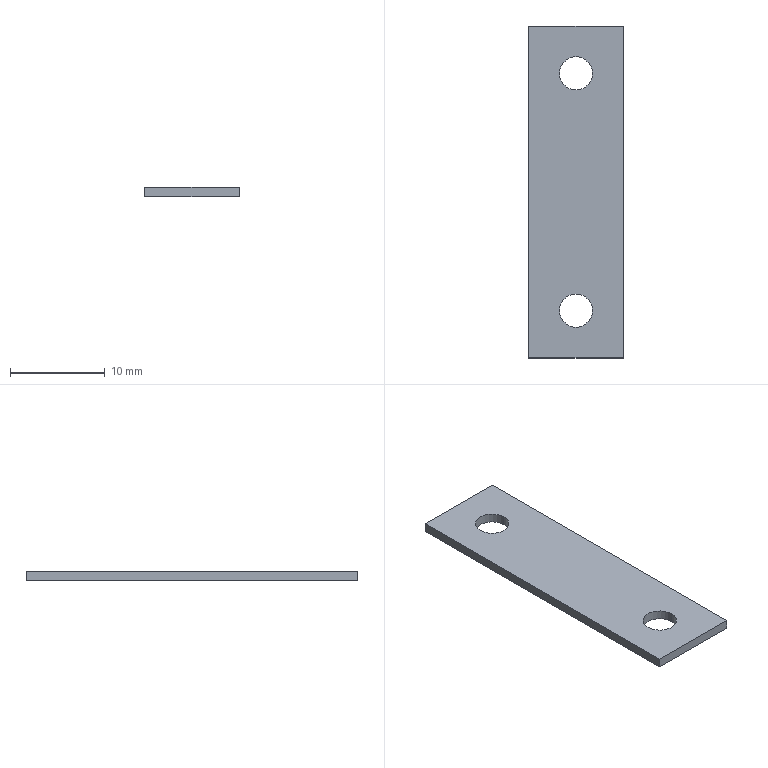Part | STEP file | D04 | 1 solid | 10 faces | box 10 x 35 x 1 mm | volume 330.758 mm3 | plane 6 | cylinder 4 | commonest cylinder face diameters 3.5 x4
STEP:
#1=CARTESIAN_POINT('',(0.,0.,0.));
#2=DIRECTION('',(0.,0.,1.));
#3=DIRECTION('',(1.,0.,0.));
#4=AXIS2_PLACEMENT_3D('',#1,#2,#3);
#5=CARTESIAN_POINT('',(1.75,-12.5,0.));
#6=VERTEX_POINT('',#5);
#7=CARTESIAN_POINT('',(1.75,-12.5,1.));
#8=VERTEX_POINT('',#7);
#9=CARTESIAN_POINT('',(1.75,-12.5,0.));
#10=DIRECTION('',(0.,0.,1.));
#11=VECTOR('',#10,1.);
#12=LINE('',#9,#11);
#13=CARTESIAN_POINT('',(0.,-12.5,0.));
#14=DIRECTION('',(0.,0.,1.));
#15=DIRECTION('',(1.,0.,0.));
#16=AXIS2_PLACEMENT_3D('',#13,#14,#15);
#17=CYLINDRICAL_SURFACE('',#16,1.75);
#18=CARTESIAN_POINT('',(6.283,0.));
#19=DIRECTION('',(0.,1.));
#20=VECTOR('',#19,1.);
#21=LINE('',#18,#20);
#22=(GEOMETRIC_REPRESENTATION_CONTEXT(2)PARAMETRIC_REPRESENTATION_CONTEXT()REPRESENTATION_CONTEXT('',''));
#23=DEFINITIONAL_REPRESENTATION('',(#21),#22);
#24=PCURVE('',#17,#23);
#25=CARTESIAN_POINT('',(0.,-12.5,0.));
#26=DIRECTION('',(0.,0.,1.));
#27=DIRECTION('',(1.,0.,0.));
#28=AXIS2_PLACEMENT_3D('',#25,#26,#27);
#29=CYLINDRICAL_SURFACE('',#28,1.75);
#30=CARTESIAN_POINT('',(0.,0.));
#31=DIRECTION('',(0.,1.));
#32=VECTOR('',#31,1.);
#33=LINE('',#30,#32);
#34=(GEOMETRIC_REPRESENTATION_CONTEXT(2)PARAMETRIC_REPRESENTATION_CONTEXT()REPRESENTATION_CONTEXT('',''));
#35=DEFINITIONAL_REPRESENTATION('',(#33),#34);
#36=PCURVE('',#29,#35);
#37=SURFACE_CURVE('',#12,(#24,#36),.PCURVE_S1.);
#38=EDGE_CURVE('',#6,#8,#37,.T.);
#39=ORIENTED_EDGE('',*,*,#38,.T.);
#40=CARTESIAN_POINT('',(-1.75,-12.5,1.));
#41=VERTEX_POINT('',#40);
#42=CARTESIAN_POINT('',(0.,-12.5,1.));
#43=DIRECTION('',(0.,0.,1.));
#44=DIRECTION('',(1.,0.,0.));
#45=AXIS2_PLACEMENT_3D('',#42,#43,#44);
#46=CIRCLE('',#45,1.75);
#47=CARTESIAN_POINT('',(0.,1.));
#48=DIRECTION('',(1.,0.));
#49=VECTOR('',#48,1.);
#50=LINE('',#47,#49);
#51=(GEOMETRIC_REPRESENTATION_CONTEXT(2)PARAMETRIC_REPRESENTATION_CONTEXT()REPRESENTATION_CONTEXT('',''));
#52=DEFINITIONAL_REPRESENTATION('',(#50),#51);
#53=PCURVE('',#17,#52);
#54=CARTESIAN_POINT('',(0.,0.,1.));
#55=DIRECTION('',(0.,0.,1.));
#56=DIRECTION('',(1.,0.,0.));
#57=AXIS2_PLACEMENT_3D('',#54,#55,#56);
#58=PLANE('',#57);
#59=CARTESIAN_POINT('',(0.,-12.5));
#60=DIRECTION('',(1.,0.));
#61=AXIS2_PLACEMENT_2D('',#59,#60);
#62=CIRCLE('',#61,1.75);
#63=(GEOMETRIC_REPRESENTATION_CONTEXT(2)PARAMETRIC_REPRESENTATION_CONTEXT()REPRESENTATION_CONTEXT('',''));
#64=DEFINITIONAL_REPRESENTATION('',(#62),#63);
#65=PCURVE('',#58,#64);
#66=SURFACE_CURVE('',#46,(#53,#65),.PCURVE_S1.);
#67=EDGE_CURVE('',#41,#8,#66,.T.);
#68=ORIENTED_EDGE('',*,*,#67,.F.);
#69=CARTESIAN_POINT('',(-1.75,-12.5,0.));
#70=VERTEX_POINT('',#69);
#71=CARTESIAN_POINT('',(-1.75,-12.5,0.));
#72=DIRECTION('',(0.,0.,1.));
#73=VECTOR('',#72,1.);
#74=LINE('',#71,#73);
#75=CARTESIAN_POINT('',(3.142,0.));
#76=DIRECTION('',(0.,1.));
#77=VECTOR('',#76,1.);
#78=LINE('',#75,#77);
#79=(GEOMETRIC_REPRESENTATION_CONTEXT(2)PARAMETRIC_REPRESENTATION_CONTEXT()REPRESENTATION_CONTEXT('',''));
#80=DEFINITIONAL_REPRESENTATION('',(#78),#79);
#81=PCURVE('',#17,#80);
#82=CARTESIAN_POINT('',(3.142,0.));
#83=DIRECTION('',(0.,1.));
#84=VECTOR('',#83,1.);
#85=LINE('',#82,#84);
#86=(GEOMETRIC_REPRESENTATION_CONTEXT(2)PARAMETRIC_REPRESENTATION_CONTEXT()REPRESENTATION_CONTEXT('',''));
#87=DEFINITIONAL_REPRESENTATION('',(#85),#86);
#88=PCURVE('',#29,#87);
#89=SURFACE_CURVE('',#74,(#81,#88),.PCURVE_S1.);
#90=EDGE_CURVE('',#70,#41,#89,.T.);
#91=ORIENTED_EDGE('',*,*,#90,.F.);
#92=CARTESIAN_POINT('',(0.,-12.5,0.));
#93=DIRECTION('',(0.,0.,1.));
#94=DIRECTION('',(1.,0.,0.));
#95=AXIS2_PLACEMENT_3D('',#92,#93,#94);
#96=CIRCLE('',#95,1.75);
#97=CARTESIAN_POINT('',(0.,0.));
#98=DIRECTION('',(1.,0.));
#99=VECTOR('',#98,1.);
#100=LINE('',#97,#99);
#101=(GEOMETRIC_REPRESENTATION_CONTEXT(2)PARAMETRIC_REPRESENTATION_CONTEXT()REPRESENTATION_CONTEXT('',''));
#102=DEFINITIONAL_REPRESENTATION('',(#100),#101);
#103=PCURVE('',#17,#102);
#104=CARTESIAN_POINT('',(0.,0.,0.));
#105=DIRECTION('',(0.,0.,1.));
#106=DIRECTION('',(1.,0.,0.));
#107=AXIS2_PLACEMENT_3D('',#104,#105,#106);
#108=PLANE('',#107);
#109=CARTESIAN_POINT('',(0.,-12.5));
#110=DIRECTION('',(1.,0.));
#111=AXIS2_PLACEMENT_2D('',#109,#110);
#112=CIRCLE('',#111,1.75);
#113=(GEOMETRIC_REPRESENTATION_CONTEXT(2)PARAMETRIC_REPRESENTATION_CONTEXT()REPRESENTATION_CONTEXT('',''));
#114=DEFINITIONAL_REPRESENTATION('',(#112),#113);
#115=PCURVE('',#108,#114);
#116=SURFACE_CURVE('',#96,(#103,#115),.PCURVE_S1.);
#117=EDGE_CURVE('',#70,#6,#116,.T.);
#118=ORIENTED_EDGE('',*,*,#117,.T.);
#119=EDGE_LOOP('',(#39,#68,#91,#118));
#120=FACE_BOUND('',#119,.F.);
#121=ADVANCED_FACE('',(#120),#17,.F.);
#122=CARTESIAN_POINT('',(1.75,12.5,0.));
#123=VERTEX_POINT('',#122);
#124=CARTESIAN_POINT('',(1.75,12.5,1.));
#125=VERTEX_POINT('',#124);
#126=CARTESIAN_POINT('',(1.75,12.5,0.));
#127=DIRECTION('',(0.,0.,1.));
#128=VECTOR('',#127,1.);
#129=LINE('',#126,#128);
#130=CARTESIAN_POINT('',(0.,12.5,0.));
#131=DIRECTION('',(0.,0.,1.));
#132=DIRECTION('',(1.,0.,0.));
#133=AXIS2_PLACEMENT_3D('',#130,#131,#132);
#134=CYLINDRICAL_SURFACE('',#133,1.75);
#135=CARTESIAN_POINT('',(6.283,0.));
#136=DIRECTION('',(0.,1.));
#137=VECTOR('',#136,1.);
#138=LINE('',#135,#137);
#139=(GEOMETRIC_REPRESENTATION_CONTEXT(2)PARAMETRIC_REPRESENTATION_CONTEXT()REPRESENTATION_CONTEXT('',''));
#140=DEFINITIONAL_REPRESENTATION('',(#138),#139);
#141=PCURVE('',#134,#140);
#142=CARTESIAN_POINT('',(0.,12.5,0.));
#143=DIRECTION('',(0.,0.,1.));
#144=DIRECTION('',(1.,0.,0.));
#145=AXIS2_PLACEMENT_3D('',#142,#143,#144);
#146=CYLINDRICAL_SURFACE('',#145,1.75);
#147=CARTESIAN_POINT('',(0.,0.));
#148=DIRECTION('',(0.,1.));
#149=VECTOR('',#148,1.);
#150=LINE('',#147,#149);
#151=(GEOMETRIC_REPRESENTATION_CONTEXT(2)PARAMETRIC_REPRESENTATION_CONTEXT()REPRESENTATION_CONTEXT('',''));
#152=DEFINITIONAL_REPRESENTATION('',(#150),#151);
#153=PCURVE('',#146,#152);
#154=SURFACE_CURVE('',#129,(#141,#153),.PCURVE_S1.);
#155=EDGE_CURVE('',#123,#125,#154,.T.);
#156=ORIENTED_EDGE('',*,*,#155,.T.);
#157=CARTESIAN_POINT('',(-1.75,12.5,1.));
#158=VERTEX_POINT('',#157);
#159=CARTESIAN_POINT('',(0.,12.5,1.));
#160=DIRECTION('',(0.,0.,1.));
#161=DIRECTION('',(1.,0.,0.));
#162=AXIS2_PLACEMENT_3D('',#159,#160,#161);
#163=CIRCLE('',#162,1.75);
#164=CARTESIAN_POINT('',(0.,1.));
#165=DIRECTION('',(1.,0.));
#166=VECTOR('',#165,1.);
#167=LINE('',#164,#166);
#168=(GEOMETRIC_REPRESENTATION_CONTEXT(2)PARAMETRIC_REPRESENTATION_CONTEXT()REPRESENTATION_CONTEXT('',''));
#169=DEFINITIONAL_REPRESENTATION('',(#167),#168);
#170=PCURVE('',#134,#169);
#171=CARTESIAN_POINT('',(0.,12.5));
#172=DIRECTION('',(1.,0.));
#173=AXIS2_PLACEMENT_2D('',#171,#172);
#174=CIRCLE('',#173,1.75);
#175=(GEOMETRIC_REPRESENTATION_CONTEXT(2)PARAMETRIC_REPRESENTATION_CONTEXT()REPRESENTATION_CONTEXT('',''));
#176=DEFINITIONAL_REPRESENTATION('',(#174),#175);
#177=PCURVE('',#58,#176);
#178=SURFACE_CURVE('',#163,(#170,#177),.PCURVE_S1.);
#179=EDGE_CURVE('',#158,#125,#178,.T.);
#180=ORIENTED_EDGE('',*,*,#179,.F.);
#181=CARTESIAN_POINT('',(-1.75,12.5,0.));
#182=VERTEX_POINT('',#181);
#183=CARTESIAN_POINT('',(-1.75,12.5,0.));
#184=DIRECTION('',(0.,0.,1.));
#185=VECTOR('',#184,1.);
#186=LINE('',#183,#185);
#187=CARTESIAN_POINT('',(3.142,0.));
#188=DIRECTION('',(0.,1.));
#189=VECTOR('',#188,1.);
#190=LINE('',#187,#189);
#191=(GEOMETRIC_REPRESENTATION_CONTEXT(2)PARAMETRIC_REPRESENTATION_CONTEXT()REPRESENTATION_CONTEXT('',''));
#192=DEFINITIONAL_REPRESENTATION('',(#190),#191);
#193=PCURVE('',#134,#192);
#194=CARTESIAN_POINT('',(3.142,0.));
#195=DIRECTION('',(0.,1.));
#196=VECTOR('',#195,1.);
#197=LINE('',#194,#196);
#198=(GEOMETRIC_REPRESENTATION_CONTEXT(2)PARAMETRIC_REPRESENTATION_CONTEXT()REPRESENTATION_CONTEXT('',''));
#199=DEFINITIONAL_REPRESENTATION('',(#197),#198);
#200=PCURVE('',#146,#199);
#201=SURFACE_CURVE('',#186,(#193,#200),.PCURVE_S1.);
#202=EDGE_CURVE('',#182,#158,#201,.T.);
#203=ORIENTED_EDGE('',*,*,#202,.F.);
#204=CARTESIAN_POINT('',(0.,12.5,0.));
#205=DIRECTION('',(0.,0.,1.));
#206=DIRECTION('',(1.,0.,0.));
#207=AXIS2_PLACEMENT_3D('',#204,#205,#206);
#208=CIRCLE('',#207,1.75);
#209=CARTESIAN_POINT('',(0.,0.));
#210=DIRECTION('',(1.,0.));
#211=VECTOR('',#210,1.);
#212=LINE('',#209,#211);
#213=(GEOMETRIC_REPRESENTATION_CONTEXT(2)PARAMETRIC_REPRESENTATION_CONTEXT()REPRESENTATION_CONTEXT('',''));
#214=DEFINITIONAL_REPRESENTATION('',(#212),#213);
#215=PCURVE('',#134,#214);
#216=CARTESIAN_POINT('',(0.,12.5));
#217=DIRECTION('',(1.,0.));
#218=AXIS2_PLACEMENT_2D('',#216,#217);
#219=CIRCLE('',#218,1.75);
#220=(GEOMETRIC_REPRESENTATION_CONTEXT(2)PARAMETRIC_REPRESENTATION_CONTEXT()REPRESENTATION_CONTEXT('',''));
#221=DEFINITIONAL_REPRESENTATION('',(#219),#220);
#222=PCURVE('',#108,#221);
#223=SURFACE_CURVE('',#208,(#215,#222),.PCURVE_S1.);
#224=EDGE_CURVE('',#182,#123,#223,.T.);
#225=ORIENTED_EDGE('',*,*,#224,.T.);
#226=EDGE_LOOP('',(#156,#180,#203,#225));
#227=FACE_BOUND('',#226,.F.);
#228=ADVANCED_FACE('',(#227),#134,.F.);
#229=CARTESIAN_POINT('',(5.,-17.5,0.));
#230=VERTEX_POINT('',#229);
#231=CARTESIAN_POINT('',(5.,17.5,0.));
#232=VERTEX_POINT('',#231);
#233=CARTESIAN_POINT('',(5.,17.5,0.));
#234=DIRECTION('',(0.,1.,0.));
#235=VECTOR('',#234,1.);
#236=LINE('',#233,#235);
#237=CARTESIAN_POINT('',(5.,17.5,1.));
#238=DIRECTION('',(-1.,0.,0.));
#239=DIRECTION('',(0.,-1.,0.));
#240=AXIS2_PLACEMENT_3D('',#237,#238,#239);
#241=PLANE('',#240);
#242=CARTESIAN_POINT('',(0.,-1.));
#243=DIRECTION('',(-1.,0.));
#244=VECTOR('',#243,1.);
#245=LINE('',#242,#244);
#246=(GEOMETRIC_REPRESENTATION_CONTEXT(2)PARAMETRIC_REPRESENTATION_CONTEXT()REPRESENTATION_CONTEXT('',''));
#247=DEFINITIONAL_REPRESENTATION('',(#245),#246);
#248=PCURVE('',#241,#247);
#249=CARTESIAN_POINT('',(5.,17.5));
#250=DIRECTION('',(0.,1.));
#251=VECTOR('',#250,1.);
#252=LINE('',#249,#251);
#253=(GEOMETRIC_REPRESENTATION_CONTEXT(2)PARAMETRIC_REPRESENTATION_CONTEXT()REPRESENTATION_CONTEXT('',''));
#254=DEFINITIONAL_REPRESENTATION('',(#252),#253);
#255=PCURVE('',#108,#254);
#256=SURFACE_CURVE('',#236,(#248,#255),.PCURVE_S1.);
#257=EDGE_CURVE('',#230,#232,#256,.T.);
#258=ORIENTED_EDGE('',*,*,#257,.T.);
#259=CARTESIAN_POINT('',(5.,17.5,1.));
#260=VERTEX_POINT('',#259);
#261=CARTESIAN_POINT('',(5.,17.5,1.));
#262=DIRECTION('',(0.,0.,-1.));
#263=VECTOR('',#262,1.);
#264=LINE('',#261,#263);
#265=CARTESIAN_POINT('',(0.,0.));
#266=DIRECTION('',(0.,-1.));
#267=VECTOR('',#266,1.);
#268=LINE('',#265,#267);
#269=(GEOMETRIC_REPRESENTATION_CONTEXT(2)PARAMETRIC_REPRESENTATION_CONTEXT()REPRESENTATION_CONTEXT('',''));
#270=DEFINITIONAL_REPRESENTATION('',(#268),#269);
#271=PCURVE('',#241,#270);
#272=CARTESIAN_POINT('',(-5.,17.5,1.));
#273=DIRECTION('',(0.,-1.,0.));
#274=DIRECTION('',(0.,0.,-1.));
#275=AXIS2_PLACEMENT_3D('',#272,#273,#274);
#276=PLANE('',#275);
#277=CARTESIAN_POINT('',(0.,10.));
#278=DIRECTION('',(1.,0.));
#279=VECTOR('',#278,1.);
#280=LINE('',#277,#279);
#281=(GEOMETRIC_REPRESENTATION_CONTEXT(2)PARAMETRIC_REPRESENTATION_CONTEXT()REPRESENTATION_CONTEXT('',''));
#282=DEFINITIONAL_REPRESENTATION('',(#280),#281);
#283=PCURVE('',#276,#282);
#284=SURFACE_CURVE('',#264,(#271,#283),.PCURVE_S1.);
#285=EDGE_CURVE('',#260,#232,#284,.T.);
#286=ORIENTED_EDGE('',*,*,#285,.F.);
#287=CARTESIAN_POINT('',(5.,-17.5,1.));
#288=VERTEX_POINT('',#287);
#289=CARTESIAN_POINT('',(5.,17.5,1.));
#290=DIRECTION('',(0.,1.,0.));
#291=VECTOR('',#290,1.);
#292=LINE('',#289,#291);
#293=CARTESIAN_POINT('',(0.,0.));
#294=DIRECTION('',(-1.,0.));
#295=VECTOR('',#294,1.);
#296=LINE('',#293,#295);
#297=(GEOMETRIC_REPRESENTATION_CONTEXT(2)PARAMETRIC_REPRESENTATION_CONTEXT()REPRESENTATION_CONTEXT('',''));
#298=DEFINITIONAL_REPRESENTATION('',(#296),#297);
#299=PCURVE('',#241,#298);
#300=CARTESIAN_POINT('',(5.,17.5));
#301=DIRECTION('',(0.,1.));
#302=VECTOR('',#301,1.);
#303=LINE('',#300,#302);
#304=(GEOMETRIC_REPRESENTATION_CONTEXT(2)PARAMETRIC_REPRESENTATION_CONTEXT()REPRESENTATION_CONTEXT('',''));
#305=DEFINITIONAL_REPRESENTATION('',(#303),#304);
#306=PCURVE('',#58,#305);
#307=SURFACE_CURVE('',#292,(#299,#306),.PCURVE_S1.);
#308=EDGE_CURVE('',#288,#260,#307,.T.);
#309=ORIENTED_EDGE('',*,*,#308,.F.);
#310=CARTESIAN_POINT('',(5.,-17.5,1.));
#311=DIRECTION('',(0.,0.,-1.));
#312=VECTOR('',#311,1.);
#313=LINE('',#310,#312);
#314=CARTESIAN_POINT('',(35.,0.));
#315=DIRECTION('',(0.,-1.));
#316=VECTOR('',#315,1.);
#317=LINE('',#314,#316);
#318=(GEOMETRIC_REPRESENTATION_CONTEXT(2)PARAMETRIC_REPRESENTATION_CONTEXT()REPRESENTATION_CONTEXT('',''));
#319=DEFINITIONAL_REPRESENTATION('',(#317),#318);
#320=PCURVE('',#241,#319);
#321=CARTESIAN_POINT('',(-5.,-17.5,1.));
#322=DIRECTION('',(0.,1.,0.));
#323=DIRECTION('',(0.,0.,1.));
#324=AXIS2_PLACEMENT_3D('',#321,#322,#323);
#325=PLANE('',#324);
#326=CARTESIAN_POINT('',(0.,10.));
#327=DIRECTION('',(-1.,0.));
#328=VECTOR('',#327,1.);
#329=LINE('',#326,#328);
#330=(GEOMETRIC_REPRESENTATION_CONTEXT(2)PARAMETRIC_REPRESENTATION_CONTEXT()REPRESENTATION_CONTEXT('',''));
#331=DEFINITIONAL_REPRESENTATION('',(#329),#330);
#332=PCURVE('',#325,#331);
#333=SURFACE_CURVE('',#313,(#320,#332),.PCURVE_S1.);
#334=EDGE_CURVE('',#288,#230,#333,.T.);
#335=ORIENTED_EDGE('',*,*,#334,.T.);
#336=EDGE_LOOP('',(#258,#286,#309,#335));
#337=FACE_BOUND('',#336,.T.);
#338=ADVANCED_FACE('',(#337),#241,.F.);
#339=CARTESIAN_POINT('',(-5.,17.5,0.));
#340=VERTEX_POINT('',#339);
#341=CARTESIAN_POINT('',(-5.,17.5,0.));
#342=DIRECTION('',(-1.,0.,0.));
#343=VECTOR('',#342,1.);
#344=LINE('',#341,#343);
#345=CARTESIAN_POINT('',(1.,0.));
#346=DIRECTION('',(0.,-1.));
#347=VECTOR('',#346,1.);
#348=LINE('',#345,#347);
#349=(GEOMETRIC_REPRESENTATION_CONTEXT(2)PARAMETRIC_REPRESENTATION_CONTEXT()REPRESENTATION_CONTEXT('',''));
#350=DEFINITIONAL_REPRESENTATION('',(#348),#349);
#351=PCURVE('',#276,#350);
#352=CARTESIAN_POINT('',(-5.,17.5));
#353=DIRECTION('',(-1.,0.));
#354=VECTOR('',#353,1.);
#355=LINE('',#352,#354);
#356=(GEOMETRIC_REPRESENTATION_CONTEXT(2)PARAMETRIC_REPRESENTATION_CONTEXT()REPRESENTATION_CONTEXT('',''));
#357=DEFINITIONAL_REPRESENTATION('',(#355),#356);
#358=PCURVE('',#108,#357);
#359=SURFACE_CURVE('',#344,(#351,#358),.PCURVE_S1.);
#360=EDGE_CURVE('',#232,#340,#359,.T.);
#361=ORIENTED_EDGE('',*,*,#360,.T.);
#362=CARTESIAN_POINT('',(-5.,17.5,1.));
#363=VERTEX_POINT('',#362);
#364=CARTESIAN_POINT('',(-5.,17.5,1.));
#365=DIRECTION('',(0.,0.,-1.));
#366=VECTOR('',#365,1.);
#367=LINE('',#364,#366);
#368=CARTESIAN_POINT('',(0.,0.));
#369=DIRECTION('',(1.,0.));
#370=VECTOR('',#369,1.);
#371=LINE('',#368,#370);
#372=(GEOMETRIC_REPRESENTATION_CONTEXT(2)PARAMETRIC_REPRESENTATION_CONTEXT()REPRESENTATION_CONTEXT('',''));
#373=DEFINITIONAL_REPRESENTATION('',(#371),#372);
#374=PCURVE('',#276,#373);
#375=CARTESIAN_POINT('',(-5.,17.5,1.));
#376=DIRECTION('',(1.,0.,0.));
#377=DIRECTION('',(0.,1.,0.));
#378=AXIS2_PLACEMENT_3D('',#375,#376,#377);
#379=PLANE('',#378);
#380=CARTESIAN_POINT('',(0.,0.));
#381=DIRECTION('',(0.,-1.));
#382=VECTOR('',#381,1.);
#383=LINE('',#380,#382);
#384=(GEOMETRIC_REPRESENTATION_CONTEXT(2)PARAMETRIC_REPRESENTATION_CONTEXT()REPRESENTATION_CONTEXT('',''));
#385=DEFINITIONAL_REPRESENTATION('',(#383),#384);
#386=PCURVE('',#379,#385);
#387=SURFACE_CURVE('',#367,(#374,#386),.PCURVE_S1.);
#388=EDGE_CURVE('',#363,#340,#387,.T.);
#389=ORIENTED_EDGE('',*,*,#388,.F.);
#390=CARTESIAN_POINT('',(-5.,17.5,1.));
#391=DIRECTION('',(-1.,0.,0.));
#392=VECTOR('',#391,1.);
#393=LINE('',#390,#392);
#394=CARTESIAN_POINT('',(0.,0.));
#395=DIRECTION('',(0.,-1.));
#396=VECTOR('',#395,1.);
#397=LINE('',#394,#396);
#398=(GEOMETRIC_REPRESENTATION_CONTEXT(2)PARAMETRIC_REPRESENTATION_CONTEXT()REPRESENTATION_CONTEXT('',''));
#399=DEFINITIONAL_REPRESENTATION('',(#397),#398);
#400=PCURVE('',#276,#399);
#401=CARTESIAN_POINT('',(-5.,17.5));
#402=DIRECTION('',(-1.,0.));
#403=VECTOR('',#402,1.);
#404=LINE('',#401,#403);
#405=(GEOMETRIC_REPRESENTATION_CONTEXT(2)PARAMETRIC_REPRESENTATION_CONTEXT()REPRESENTATION_CONTEXT('',''));
#406=DEFINITIONAL_REPRESENTATION('',(#404),#405);
#407=PCURVE('',#58,#406);
#408=SURFACE_CURVE('',#393,(#400,#407),.PCURVE_S1.);
#409=EDGE_CURVE('',#260,#363,#408,.T.);
#410=ORIENTED_EDGE('',*,*,#409,.F.);
#411=ORIENTED_EDGE('',*,*,#285,.T.);
#412=EDGE_LOOP('',(#361,#389,#410,#411));
#413=FACE_BOUND('',#412,.T.);
#414=ADVANCED_FACE('',(#413),#276,.F.);
#415=CARTESIAN_POINT('',(-5.,-17.5,0.));
#416=VERTEX_POINT('',#415);
#417=CARTESIAN_POINT('',(-5.,17.5,0.));
#418=DIRECTION('',(0.,-1.,0.));
#419=VECTOR('',#418,1.);
#420=LINE('',#417,#419);
#421=CARTESIAN_POINT('',(0.,-1.));
#422=DIRECTION('',(-1.,0.));
#423=VECTOR('',#422,1.);
#424=LINE('',#421,#423);
#425=(GEOMETRIC_REPRESENTATION_CONTEXT(2)PARAMETRIC_REPRESENTATION_CONTEXT()REPRESENTATION_CONTEXT('',''));
#426=DEFINITIONAL_REPRESENTATION('',(#424),#425);
#427=PCURVE('',#379,#426);
#428=CARTESIAN_POINT('',(-5.,17.5));
#429=DIRECTION('',(0.,-1.));
#430=VECTOR('',#429,1.);
#431=LINE('',#428,#430);
#432=(GEOMETRIC_REPRESENTATION_CONTEXT(2)PARAMETRIC_REPRESENTATION_CONTEXT()REPRESENTATION_CONTEXT('',''));
#433=DEFINITIONAL_REPRESENTATION('',(#431),#432);
#434=PCURVE('',#108,#433);
#435=SURFACE_CURVE('',#420,(#427,#434),.PCURVE_S1.);
#436=EDGE_CURVE('',#340,#416,#435,.T.);
#437=ORIENTED_EDGE('',*,*,#436,.T.);
#438=CARTESIAN_POINT('',(-5.,-17.5,1.));
#439=VERTEX_POINT('',#438);
#440=CARTESIAN_POINT('',(-5.,-17.5,1.));
#441=DIRECTION('',(0.,0.,-1.));
#442=VECTOR('',#441,1.);
#443=LINE('',#440,#442);
#444=CARTESIAN_POINT('',(-35.,0.));
#445=DIRECTION('',(0.,-1.));
#446=VECTOR('',#445,1.);
#447=LINE('',#444,#446);
#448=(GEOMETRIC_REPRESENTATION_CONTEXT(2)PARAMETRIC_REPRESENTATION_CONTEXT()REPRESENTATION_CONTEXT('',''));
#449=DEFINITIONAL_REPRESENTATION('',(#447),#448);
#450=PCURVE('',#379,#449);
#451=CARTESIAN_POINT('',(0.,0.));
#452=DIRECTION('',(-1.,0.));
#453=VECTOR('',#452,1.);
#454=LINE('',#451,#453);
#455=(GEOMETRIC_REPRESENTATION_CONTEXT(2)PARAMETRIC_REPRESENTATION_CONTEXT()REPRESENTATION_CONTEXT('',''));
#456=DEFINITIONAL_REPRESENTATION('',(#454),#455);
#457=PCURVE('',#325,#456);
#458=SURFACE_CURVE('',#443,(#450,#457),.PCURVE_S1.);
#459=EDGE_CURVE('',#439,#416,#458,.T.);
#460=ORIENTED_EDGE('',*,*,#459,.F.);
#461=CARTESIAN_POINT('',(-5.,17.5,1.));
#462=DIRECTION('',(0.,-1.,0.));
#463=VECTOR('',#462,1.);
#464=LINE('',#461,#463);
#465=CARTESIAN_POINT('',(0.,0.));
#466=DIRECTION('',(-1.,0.));
#467=VECTOR('',#466,1.);
#468=LINE('',#465,#467);
#469=(GEOMETRIC_REPRESENTATION_CONTEXT(2)PARAMETRIC_REPRESENTATION_CONTEXT()REPRESENTATION_CONTEXT('',''));
#470=DEFINITIONAL_REPRESENTATION('',(#468),#469);
#471=PCURVE('',#379,#470);
#472=CARTESIAN_POINT('',(-5.,17.5));
#473=DIRECTION('',(0.,-1.));
#474=VECTOR('',#473,1.);
#475=LINE('',#472,#474);
#476=(GEOMETRIC_REPRESENTATION_CONTEXT(2)PARAMETRIC_REPRESENTATION_CONTEXT()REPRESENTATION_CONTEXT('',''));
#477=DEFINITIONAL_REPRESENTATION('',(#475),#476);
#478=PCURVE('',#58,#477);
#479=SURFACE_CURVE('',#464,(#471,#478),.PCURVE_S1.);
#480=EDGE_CURVE('',#363,#439,#479,.T.);
#481=ORIENTED_EDGE('',*,*,#480,.F.);
#482=ORIENTED_EDGE('',*,*,#388,.T.);
#483=EDGE_LOOP('',(#437,#460,#481,#482));
#484=FACE_BOUND('',#483,.T.);
#485=ADVANCED_FACE('',(#484),#379,.F.);
#486=CARTESIAN_POINT('',(-5.,-17.5,0.));
#487=DIRECTION('',(1.,0.,0.));
#488=VECTOR('',#487,1.);
#489=LINE('',#486,#488);
#490=CARTESIAN_POINT('',(-1.,0.));
#491=DIRECTION('',(0.,1.));
#492=VECTOR('',#491,1.);
#493=LINE('',#490,#492);
#494=(GEOMETRIC_REPRESENTATION_CONTEXT(2)PARAMETRIC_REPRESENTATION_CONTEXT()REPRESENTATION_CONTEXT('',''));
#495=DEFINITIONAL_REPRESENTATION('',(#493),#494);
#496=PCURVE('',#325,#495);
#497=CARTESIAN_POINT('',(-5.,-17.5));
#498=DIRECTION('',(1.,0.));
#499=VECTOR('',#498,1.);
#500=LINE('',#497,#499);
#501=(GEOMETRIC_REPRESENTATION_CONTEXT(2)PARAMETRIC_REPRESENTATION_CONTEXT()REPRESENTATION_CONTEXT('',''));
#502=DEFINITIONAL_REPRESENTATION('',(#500),#501);
#503=PCURVE('',#108,#502);
#504=SURFACE_CURVE('',#489,(#496,#503),.PCURVE_S1.);
#505=EDGE_CURVE('',#416,#230,#504,.T.);
#506=ORIENTED_EDGE('',*,*,#505,.T.);
#507=ORIENTED_EDGE('',*,*,#334,.F.);
#508=CARTESIAN_POINT('',(-5.,-17.5,1.));
#509=DIRECTION('',(1.,0.,0.));
#510=VECTOR('',#509,1.);
#511=LINE('',#508,#510);
#512=CARTESIAN_POINT('',(0.,0.));
#513=DIRECTION('',(0.,1.));
#514=VECTOR('',#513,1.);
#515=LINE('',#512,#514);
#516=(GEOMETRIC_REPRESENTATION_CONTEXT(2)PARAMETRIC_REPRESENTATION_CONTEXT()REPRESENTATION_CONTEXT('',''));
#517=DEFINITIONAL_REPRESENTATION('',(#515),#516);
#518=PCURVE('',#325,#517);
#519=CARTESIAN_POINT('',(-5.,-17.5));
#520=DIRECTION('',(1.,0.));
#521=VECTOR('',#520,1.);
#522=LINE('',#519,#521);
#523=(GEOMETRIC_REPRESENTATION_CONTEXT(2)PARAMETRIC_REPRESENTATION_CONTEXT()REPRESENTATION_CONTEXT('',''));
#524=DEFINITIONAL_REPRESENTATION('',(#522),#523);
#525=PCURVE('',#58,#524);
#526=SURFACE_CURVE('',#511,(#518,#525),.PCURVE_S1.);
#527=EDGE_CURVE('',#439,#288,#526,.T.);
#528=ORIENTED_EDGE('',*,*,#527,.F.);
#529=ORIENTED_EDGE('',*,*,#459,.T.);
#530=EDGE_LOOP('',(#506,#507,#528,#529));
#531=FACE_BOUND('',#530,.T.);
#532=ADVANCED_FACE('',(#531),#325,.F.);
#533=CARTESIAN_POINT('',(0.,-12.5,1.));
#534=DIRECTION('',(0.,0.,1.));
#535=DIRECTION('',(1.,0.,0.));
#536=AXIS2_PLACEMENT_3D('',#533,#534,#535);
#537=CIRCLE('',#536,1.75);
#538=CARTESIAN_POINT('',(0.,-12.5));
#539=DIRECTION('',(1.,0.));
#540=AXIS2_PLACEMENT_2D('',#538,#539);
#541=CIRCLE('',#540,1.75);
#542=(GEOMETRIC_REPRESENTATION_CONTEXT(2)PARAMETRIC_REPRESENTATION_CONTEXT()REPRESENTATION_CONTEXT('',''));
#543=DEFINITIONAL_REPRESENTATION('',(#541),#542);
#544=PCURVE('',#58,#543);
#545=CARTESIAN_POINT('',(0.,1.));
#546=DIRECTION('',(1.,0.));
#547=VECTOR('',#546,1.);
#548=LINE('',#545,#547);
#549=(GEOMETRIC_REPRESENTATION_CONTEXT(2)PARAMETRIC_REPRESENTATION_CONTEXT()REPRESENTATION_CONTEXT('',''));
#550=DEFINITIONAL_REPRESENTATION('',(#548),#549);
#551=PCURVE('',#29,#550);
#552=SURFACE_CURVE('',#537,(#544,#551),.PCURVE_S1.);
#553=EDGE_CURVE('',#8,#41,#552,.T.);
#554=ORIENTED_EDGE('',*,*,#553,.F.);
#555=ORIENTED_EDGE('',*,*,#67,.F.);
#556=EDGE_LOOP('',(#554,#555));
#557=FACE_BOUND('',#556,.T.);
#558=CARTESIAN_POINT('',(0.,12.5,1.));
#559=DIRECTION('',(0.,0.,1.));
#560=DIRECTION('',(1.,0.,0.));
#561=AXIS2_PLACEMENT_3D('',#558,#559,#560);
#562=CIRCLE('',#561,1.75);
#563=CARTESIAN_POINT('',(0.,12.5));
#564=DIRECTION('',(1.,0.));
#565=AXIS2_PLACEMENT_2D('',#563,#564);
#566=CIRCLE('',#565,1.75);
#567=(GEOMETRIC_REPRESENTATION_CONTEXT(2)PARAMETRIC_REPRESENTATION_CONTEXT()REPRESENTATION_CONTEXT('',''));
#568=DEFINITIONAL_REPRESENTATION('',(#566),#567);
#569=PCURVE('',#58,#568);
#570=CARTESIAN_POINT('',(0.,1.));
#571=DIRECTION('',(1.,0.));
#572=VECTOR('',#571,1.);
#573=LINE('',#570,#572);
#574=(GEOMETRIC_REPRESENTATION_CONTEXT(2)PARAMETRIC_REPRESENTATION_CONTEXT()REPRESENTATION_CONTEXT('',''));
#575=DEFINITIONAL_REPRESENTATION('',(#573),#574);
#576=PCURVE('',#146,#575);
#577=SURFACE_CURVE('',#562,(#569,#576),.PCURVE_S1.);
#578=EDGE_CURVE('',#125,#158,#577,.T.);
#579=ORIENTED_EDGE('',*,*,#578,.F.);
#580=ORIENTED_EDGE('',*,*,#179,.F.);
#581=EDGE_LOOP('',(#579,#580));
#582=FACE_BOUND('',#581,.T.);
#583=ORIENTED_EDGE('',*,*,#308,.T.);
#584=ORIENTED_EDGE('',*,*,#409,.T.);
#585=ORIENTED_EDGE('',*,*,#480,.T.);
#586=ORIENTED_EDGE('',*,*,#527,.T.);
#587=EDGE_LOOP('',(#583,#584,#585,#586));
#588=FACE_BOUND('',#587,.T.);
#589=ADVANCED_FACE('',(#557,#582,#588),#58,.T.);
#590=CARTESIAN_POINT('',(0.,-12.5,0.));
#591=DIRECTION('',(0.,0.,1.));
#592=DIRECTION('',(1.,0.,0.));
#593=AXIS2_PLACEMENT_3D('',#590,#591,#592);
#594=CIRCLE('',#593,1.75);
#595=CARTESIAN_POINT('',(0.,-12.5));
#596=DIRECTION('',(1.,0.));
#597=AXIS2_PLACEMENT_2D('',#595,#596);
#598=CIRCLE('',#597,1.75);
#599=(GEOMETRIC_REPRESENTATION_CONTEXT(2)PARAMETRIC_REPRESENTATION_CONTEXT()REPRESENTATION_CONTEXT('',''));
#600=DEFINITIONAL_REPRESENTATION('',(#598),#599);
#601=PCURVE('',#108,#600);
#602=CARTESIAN_POINT('',(0.,0.));
#603=DIRECTION('',(1.,0.));
#604=VECTOR('',#603,1.);
#605=LINE('',#602,#604);
#606=(GEOMETRIC_REPRESENTATION_CONTEXT(2)PARAMETRIC_REPRESENTATION_CONTEXT()REPRESENTATION_CONTEXT('',''));
#607=DEFINITIONAL_REPRESENTATION('',(#605),#606);
#608=PCURVE('',#29,#607);
#609=SURFACE_CURVE('',#594,(#601,#608),.PCURVE_S1.);
#610=EDGE_CURVE('',#6,#70,#609,.T.);
#611=ORIENTED_EDGE('',*,*,#610,.T.);
#612=ORIENTED_EDGE('',*,*,#117,.T.);
#613=EDGE_LOOP('',(#611,#612));
#614=FACE_BOUND('',#613,.T.);
#615=CARTESIAN_POINT('',(0.,12.5,0.));
#616=DIRECTION('',(0.,0.,1.));
#617=DIRECTION('',(1.,0.,0.));
#618=AXIS2_PLACEMENT_3D('',#615,#616,#617);
#619=CIRCLE('',#618,1.75);
#620=CARTESIAN_POINT('',(0.,12.5));
#621=DIRECTION('',(1.,0.));
#622=AXIS2_PLACEMENT_2D('',#620,#621);
#623=CIRCLE('',#622,1.75);
#624=(GEOMETRIC_REPRESENTATION_CONTEXT(2)PARAMETRIC_REPRESENTATION_CONTEXT()REPRESENTATION_CONTEXT('',''));
#625=DEFINITIONAL_REPRESENTATION('',(#623),#624);
#626=PCURVE('',#108,#625);
#627=CARTESIAN_POINT('',(0.,0.));
#628=DIRECTION('',(1.,0.));
#629=VECTOR('',#628,1.);
#630=LINE('',#627,#629);
#631=(GEOMETRIC_REPRESENTATION_CONTEXT(2)PARAMETRIC_REPRESENTATION_CONTEXT()REPRESENTATION_CONTEXT('',''));
#632=DEFINITIONAL_REPRESENTATION('',(#630),#631);
#633=PCURVE('',#146,#632);
#634=SURFACE_CURVE('',#619,(#626,#633),.PCURVE_S1.);
#635=EDGE_CURVE('',#123,#182,#634,.T.);
#636=ORIENTED_EDGE('',*,*,#635,.T.);
#637=ORIENTED_EDGE('',*,*,#224,.T.);
#638=EDGE_LOOP('',(#636,#637));
#639=FACE_BOUND('',#638,.T.);
#640=ORIENTED_EDGE('',*,*,#257,.F.);
#641=ORIENTED_EDGE('',*,*,#505,.F.);
#642=ORIENTED_EDGE('',*,*,#436,.F.);
#643=ORIENTED_EDGE('',*,*,#360,.F.);
#644=EDGE_LOOP('',(#640,#641,#642,#643));
#645=FACE_BOUND('',#644,.T.);
#646=ADVANCED_FACE('',(#614,#639,#645),#108,.F.);
#647=ORIENTED_EDGE('',*,*,#578,.F.);
#648=ORIENTED_EDGE('',*,*,#155,.F.);
#649=ORIENTED_EDGE('',*,*,#635,.T.);
#650=ORIENTED_EDGE('',*,*,#202,.T.);
#651=EDGE_LOOP('',(#647,#648,#649,#650));
#652=FACE_BOUND('',#651,.F.);
#653=ADVANCED_FACE('',(#652),#146,.F.);
#654=ORIENTED_EDGE('',*,*,#553,.F.);
#655=ORIENTED_EDGE('',*,*,#38,.F.);
#656=ORIENTED_EDGE('',*,*,#610,.T.);
#657=ORIENTED_EDGE('',*,*,#90,.T.);
#658=EDGE_LOOP('',(#654,#655,#656,#657));
#659=FACE_BOUND('',#658,.F.);
#660=ADVANCED_FACE('',(#659),#29,.F.);
#661=CLOSED_SHELL('',(#121,#228,#338,#414,#485,#532,#589,#646,#653,#660));
#662=MANIFOLD_SOLID_BREP('',#661);
#663=(LENGTH_UNIT()NAMED_UNIT(*)SI_UNIT(.MILLI.,.METRE.));
#664=UNCERTAINTY_MEASURE_WITH_UNIT(LENGTH_MEASURE(0.0000001),#663,'','');
#665=(NAMED_UNIT(*)PLANE_ANGLE_UNIT()SI_UNIT($,.RADIAN.));
#666=(NAMED_UNIT(*)SI_UNIT($,.STERADIAN.)SOLID_ANGLE_UNIT());
#667=(GEOMETRIC_REPRESENTATION_CONTEXT(3)GLOBAL_UNCERTAINTY_ASSIGNED_CONTEXT((#664))GLOBAL_UNIT_ASSIGNED_CONTEXT((#663,#665,#666))REPRESENTATION_CONTEXT('',''));
#668=ADVANCED_BREP_SHAPE_REPRESENTATION('',(#4,#662),#667);